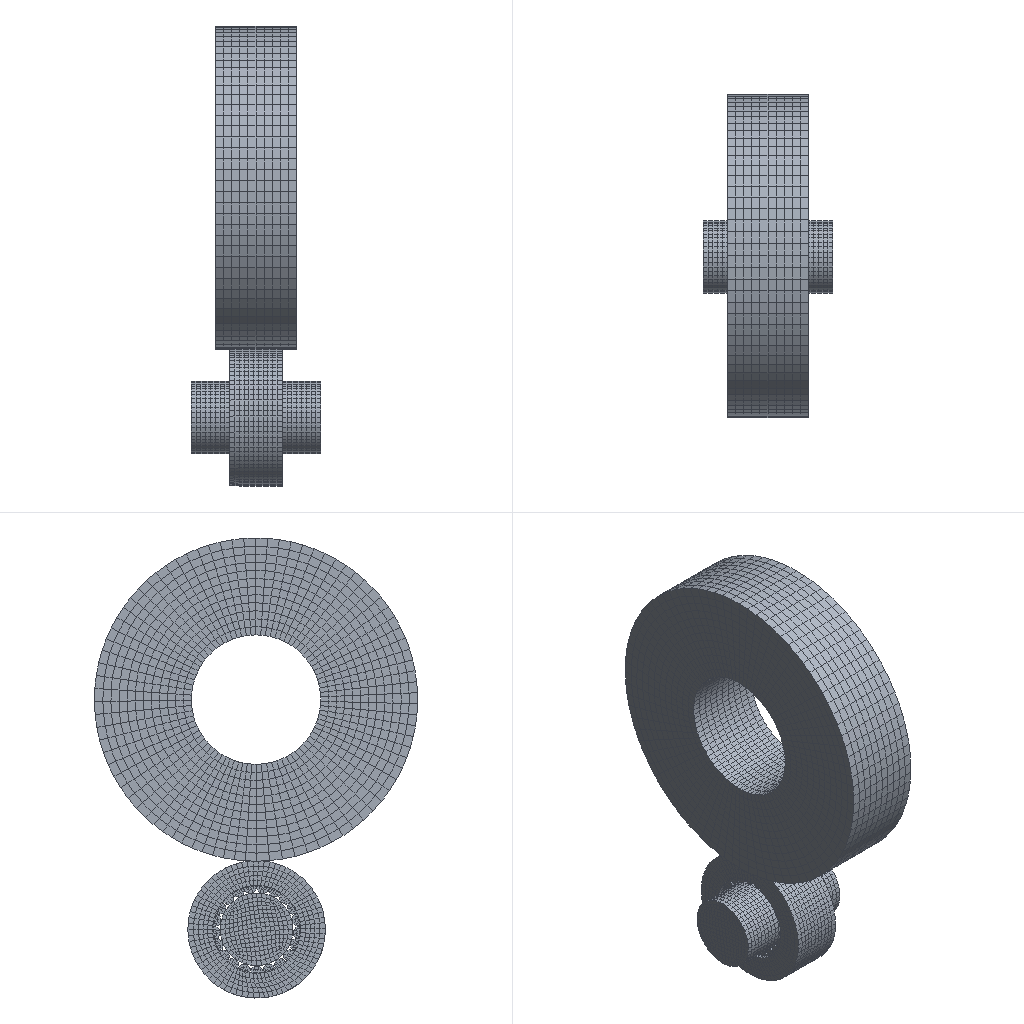Simulation study | abaqus
Set-up summary:
category,name,step,type,value,unit,region
solver,abaqus
solver,version,,,Abaqus/Explicit 2020
units,not stated in the deck,,not stated
analysis,deck,,transient,transient
load_step,Step-1,Step-1,transient
load_step,requested,,,1
mesh,nodes,,,28916
mesh,elements,,,23080
element_type,C3D8R,,solid,23080
load,load commands in deck,,count,3
bc,support commands in deck,,count,13
material,MATERIAL-1,,in results
check,setup vs results,,match,"per instance, exact: element labels, types and connectivity; labels of the nodes the elements use; coordinates of those nodes at SINGLE_PRECISION in 24 of 24 instance(s)"
Abaqus input file, long lists of numbers shortened:
*Heading
** Job name: Job-1 Model name: Model-1
** Generated by: Abaqus/CAE 2020
*Preprint, echo=NO, model=NO, history=NO, contact=NO
**
** PARTS
**
*Part, name=work-1
*Node
      1,  -7.421,    98.793,  -140.361
      2,  -7.421,   99.389,  -144.043
** (218 more lines like these left out)
*Element, type=C3D8R
  1,  17,   7,   1,   6,  39,  29,  23,  28
  2,  17,   8,   2,   7,  39,  30,  24,  29
** (142 more lines like these left out)
*Nset, nset=Set-2, generate
   1,  220,    1
*Elset, elset=Set-2, generate
   1,  144,    1
** Section: Section-1
*Solid Section, elset=Set-2, material=Material-1
,
*End Part
**
*Part, name=work-2
*Node
      1,  -7.421,   127.968,  -119.26
      2,  -7.421,   124.847,   -118.703
** (4862 more lines like these left out)
*Element, type=C3D8R
  1,   86,  140,  139,   87, 1088,  382,  383, 1089
  2,   85,  141,  140,   86, 1087,  381,  382, 1088
** (3494 more lines like these left out)
*Nset, nset=Set-2, generate
    1,  4864,     1
*Elset, elset=Set-2, generate
    1,  3496,     1
** Section: Section-1
*Solid Section, elset=Set-2, material=Material-1
,
*End Part
**
*Part, name=work-3
*Node
      1,  -7.421,   90.453,   -143.093
      2,  -7.421,    90.968,  -139.399
** (218 more lines like these left out)
*Element, type=C3D8R
  1,  17,  18,   7,   6,  39,  40,  29,  28
  2,  18,   8,   1,   7,  40,  30,  23,  29
** (142 more lines like these left out)
*Nset, nset=Set-2, generate
   1,  220,    1
*Elset, elset=Set-2, generate
   1,  144,    1
** Section: Section-1
*Solid Section, elset=Set-2, material=Material-1
,
*End Part
**
*Part, name=work-4
*Node
      1,  -7.421,   82.194,  -139.552
      2,  -7.421,   83.775,  -136.174
** (218 more lines like these left out)
*Element, type=C3D8R
  1,  17,  18,   7,   6,  39,  40,  29,  28
  2,  18,   8,   1,   7,  40,  30,  23,  29
** (142 more lines like these left out)
*Nset, nset=Set-2, generate
   1,  220,    1
*Elset, elset=Set-2, generate
   1,  144,    1
** Section: Section-1
*Solid Section, elset=Set-2, material=Material-1
,
*End Part
**
*Part, name=work-5
*Node
      1,  -7.421,   75.345,  -133.734
      2,  -7.421,   77.852,  -130.972
** (218 more lines like these left out)
*Element, type=C3D8R
  1,  17,  18,   7,   6,  39,  40,  29,  28
  2,  18,   8,   1,   7,  40,  30,  23,  29
** (142 more lines like these left out)
*Nset, nset=Set-2, generate
   1,  220,    1
*Elset, elset=Set-2, generate
   1,  144,    1
** Section: Section-1
*Solid Section, elset=Set-2, material=Material-1
,
*End Part
**
*Part, name=work-6
*Node
      1,  -7.421,   73.153,  -122.789
      2,  -7.421,   69.504,   -123.541
** (218 more lines like these left out)
*Element, type=C3D8R
  1,  17,  18,   7,   6,  39,  40,  29,  28
  2,  18,   8,   1,   7,  40,  30,  23,  29
** (142 more lines like these left out)
*Nset, nset=Set-2, generate
   1,  220,    1
*Elset, elset=Set-2, generate
   1,  144,    1
** Section: Section-1
*Solid Section, elset=Set-2, material=Material-1
,
*End Part
**
*Part, name=work-7
*Node
      1,  -7.421,   68.134,  -117.49
      2,  -7.421,   71.761,  -116.62
** (218 more lines like these left out)
*Element, type=C3D8R
  1,  17,  18,   7,   6,  39,  40,  29,  28
  2,  18,   8,   1,   7,  40,  30,  23,  29
** (142 more lines like these left out)
*Nset, nset=Set-2, generate
   1,  220,    1
*Elset, elset=Set-2, generate
   1,  144,    1
** Section: Section-1
*Solid Section, elset=Set-2, material=Material-1
,
*End Part
**
*Part, name=work-8
*Node
      1,  -7.421,   68.413,  -108.508
      2,  -7.421,   72.135,  -108.746
** (218 more lines like these left out)
*Element, type=C3D8R
  1,  17,  18,   7,   6,  39,  40,  29,  28
  2,  18,   8,   1,   7,  40,  30,  23,  29
** (142 more lines like these left out)
*Nset, nset=Set-2, generate
   1,  220,    1
*Elset, elset=Set-2, generate
   1,  144,    1
** Section: Section-1
*Solid Section, elset=Set-2, material=Material-1
,
*End Part
**
*Part, name=work-9
*Node
      1,  -7.421,   75.604,  -99.97
      2,  -7.421,   72.741,  -97.586
** (218 more lines like these left out)
*Element, type=C3D8R
  1,  17,  18,   7,   6,  39,  40,  29,  28
  2,  18,   8,   1,   7,  40,  30,  23,  29
** (142 more lines like these left out)
*Nset, nset=Set-2, generate
   1,  220,    1
*Elset, elset=Set-2, generate
   1,  144,    1
** Section: Section-1
*Solid Section, elset=Set-2, material=Material-1
,
*End Part
**
*Part, name=work-10
*Node
      1,  -7.421,   76.617,  -92.743
      2,  -7.421,   79.559,  -95.036
** (218 more lines like these left out)
*Element, type=C3D8R
  1,  17,  18,   7,   6,  39,  40,  29,  28
  2,  18,   8,   1,   7,  40,  30,  23,  29
** (142 more lines like these left out)
*Nset, nset=Set-2, generate
   1,  220,    1
*Elset, elset=Set-2, generate
   1,  144,    1
** Section: Section-1
*Solid Section, elset=Set-2, material=Material-1
,
*End Part
**
*Part, name=work-11
*Node
      1,  -7.421,   87.368,  -89.739
      2,  -7.421,   86.346,  -86.156
** (218 more lines like these left out)
*Element, type=C3D8R
  1,  17,  18,   7,   6,  39,  40,  29,  28
  2,  18,   8,   1,   7,  40,  30,  23,  29
** (142 more lines like these left out)
*Nset, nset=Set-2, generate
   1,  220,    1
*Elset, elset=Set-2, generate
   1,  144,    1
** Section: Section-1
*Solid Section, elset=Set-2, material=Material-1
,
*End Part
**
*Part, name=work-12
*Node
      1,  -7.421,   94.972,  -87.659
      2,  -7.421,   95.051,  -83.934
** (218 more lines like these left out)
*Element, type=C3D8R
  1,  17,  18,   7,   6,  39,  40,  29,  28
  2,  18,   8,   1,   7,  40,  30,  23,  29
** (142 more lines like these left out)
*Nset, nset=Set-2, generate
   1,  220,    1
*Elset, elset=Set-2, generate
   1,  144,    1
** Section: Section-1
*Solid Section, elset=Set-2, material=Material-1
,
*End Part
**
*Part, name=work-13
*Node
      1,  -7.421,   102.852,  -87.913
      2,  -7.421,   104.025,  -84.377
** (218 more lines like these left out)
*Element, type=C3D8R
  1,  17,  18,   7,   6,  39,  40,  29,  28
  2,  18,   8,   1,   7,  40,  30,  23,  29
** (142 more lines like these left out)
*Nset, nset=Set-2, generate
   1,  220,    1
*Elset, elset=Set-2, generate
   1,  144,    1
** Section: Section-1
*Solid Section, elset=Set-2, material=Material-1
,
*End Part
**
*Part, name=work-14
*Node
      1,  -7.421,   109.95,  -86.216
      2,  -7.421,   108.89,  -89.792
** (218 more lines like these left out)
*Element, type=C3D8R
  1,  17,  18,   7,   6,  39,  40,  29,  28
  2,  18,   8,   1,   7,  40,  30,  23,  29
** (142 more lines like these left out)
*Nset, nset=Set-2, generate
   1,  220,    1
*Elset, elset=Set-2, generate
   1,  144,    1
** Section: Section-1
*Solid Section, elset=Set-2, material=Material-1
,
*End Part
**
*Part, name=work-15
*Node
      1,  -7.421,   117.589,  -90.948
      2,  -7.421,   115.522,  -94.053
** (218 more lines like these left out)
*Element, type=C3D8R
  1,  17,  18,   7,   6,  39,  40,  29,  28
  2,  18,   8,   1,   7,  40,  30,  23,  29
** (142 more lines like these left out)
*Nset, nset=Set-2, generate
   1,  220,    1
*Elset, elset=Set-2, generate
   1,  144,    1
** Section: Section-1
*Solid Section, elset=Set-2, material=Material-1
,
*End Part
**
*Part, name=work-16
*Node
      1,  -7.421,   121.387,  -101.445
      2,  -7.421,   124.884,  -100.157
** (218 more lines like these left out)
*Element, type=C3D8R
  1,  17,  18,   7,   6,  39,  40,  29,  28
  2,  18,   8,   1,   7,  40,  30,  23,  29
** (142 more lines like these left out)
*Nset, nset=Set-2, generate
   1,  220,    1
*Elset, elset=Set-2, generate
   1,  144,    1
** Section: Section-1
*Solid Section, elset=Set-2, material=Material-1
,
*End Part
**
*Part, name=work-17
*Node
      1,  -7.421,   124.03,  -108.872
      2,  -7.421,    127.75,   -108.672
** (218 more lines like these left out)
*Element, type=C3D8R
  1,  17,  18,   7,   6,  39,  40,  29,  28
  2,  18,   8,   1,   7,  40,  30,  23,  29
** (142 more lines like these left out)
*Nset, nset=Set-2, generate
   1,  220,    1
*Elset, elset=Set-2, generate
   1,  144,    1
** Section: Section-1
*Solid Section, elset=Set-2, material=Material-1
,
*End Part
**
*Part, name=work-18
*Node
      1,  -7.421,   128.203,   -114.859
      2,  -7.421,   124.487,  -115.179
** (218 more lines like these left out)
*Element, type=C3D8R
  1,  17,  18,   7,   6,  39,  40,  29,  28
  2,  18,   8,   1,   7,  40,  30,  23,  29
** (142 more lines like these left out)
*Nset, nset=Set-2, generate
   1,  220,    1
*Elset, elset=Set-2, generate
   1,  144,    1
** Section: Section-1
*Solid Section, elset=Set-2, material=Material-1
,
*End Part
**
*Part, name=work-19
*Node
      1,  -7.421,   126.589,  -123.7
      2,  -7.421,    122.944,  -122.91
** (218 more lines like these left out)
*Element, type=C3D8R
  1,  17,  18,   7,   6,  39,  40,  29,  28
  2,  18,   8,   1,   7,  40,  30,  23,  29
** (142 more lines like these left out)
*Nset, nset=Set-2, generate
   1,  220,    1
*Elset, elset=Set-2, generate
   1,  144,    1
** Section: Section-1
*Solid Section, elset=Set-2, material=Material-1
,
*End Part
**
*Part, name=work-20
*Node
      1,  -7.421,   122.44,  -131.671
      2,  -7.421,   119.19,  -129.842
** (218 more lines like these left out)
*Element, type=C3D8R
  1,  17,  18,   7,   6,  39,  40,  29,  28
  2,  18,   8,   1,   7,  40,  30,  23,  29
** (142 more lines like these left out)
*Nset, nset=Set-2, generate
   1,  220,    1
*Elset, elset=Set-2, generate
   1,  144,    1
** Section: Section-1
*Solid Section, elset=Set-2, material=Material-1
,
*End Part
**
*Part, name=work-21
*Node
      1,  -7.421,   116.127,  -138.066
      2,  -7.421,   113.56,  -135.36
** (218 more lines like these left out)
*Element, type=C3D8R
  1,  17,  18,   7,   6,  39,  40,  29,  28
  2,  18,   8,   1,   7,  40,  30,  23,  29
** (142 more lines like these left out)
*Nset, nset=Set-2, generate
   1,  220,    1
*Elset, elset=Set-2, generate
   1,  144,    1
** Section: Section-1
*Solid Section, elset=Set-2, material=Material-1
,
*End Part
**
*Part, name=work-22
*Node
      1,  -7.421,    106.553,  -138.973
      2,  -7.421,   108.208,  -142.316
** (218 more lines like these left out)
*Element, type=C3D8R
  1,  17,   7,   1,   6,  39,  29,  23,  28
  2,  17,   8,   2,   7,  39,  30,  24,  29
** (142 more lines like these left out)
*Nset, nset=Set-2, generate
   1,  220,    1
*Elset, elset=Set-2, generate
   1,  144,    1
** Section: Section-1
*Solid Section, elset=Set-2, material=Material-1
,
*End Part
**
*Part, name=work-23
*Node
      1,   19.579,   98.623,  -109.942
      2,   19.579,   76.403,  -107.859
** (7418 more lines like these left out)
*Element, type=C3D8R
   1,   89,   91,    8,    7,  354,  356,  273,  272
   2,   91,   92,    9,    8,  356,  357,  274,  273
** (6478 more lines like these left out)
*Nset, nset=Set-2, generate
    1,  7420,     1
*Elset, elset=Set-2, generate
    1,  6480,     1
** Section: Section-1
*Solid Section, elset=Set-2, material=Material-1
,
*End Part
**
*Part, name=work-24
*Node
      1,  -45.421,   60.427,   41.094
      2,  -45.421,   3.444,   59.882
** (12010 more lines like these left out)
*Element, type=C3D8R
    1,    66,   235,    13,     1,  1158,  1327,  1105,  1093
    2,   235,   236,    14,    13,  1327,  1328,  1106,  1105
** (10078 more lines like these left out)
*Nset, nset=Set-2, generate
     1,  12012,      1
*Elset, elset=Set-2, generate
     1,  10080,      1
** Section: Section-1
*Solid Section, elset=Set-2, material=Material-1
,
*End Part
**
**
** ASSEMBLY
**
*Assembly, name=Assembly
**
*Instance, name=work-1-1, part=work-1
*End Instance
**
*Instance, name=work-2-1, part=work-2
*End Instance
**
*Instance, name=work-3-1, part=work-3
*End Instance
**
*Instance, name=work-4-1, part=work-4
*End Instance
**
*Instance, name=work-5-1, part=work-5
*End Instance
**
*Instance, name=work-6-1, part=work-6
*End Instance
**
*Instance, name=work-7-1, part=work-7
*End Instance
**
*Instance, name=work-8-1, part=work-8
*End Instance
**
*Instance, name=work-9-1, part=work-9
*End Instance
**
*Instance, name=work-10-1, part=work-10
*End Instance
**
*Instance, name=work-11-1, part=work-11
*End Instance
**
*Instance, name=work-12-1, part=work-12
*End Instance
**
*Instance, name=work-13-1, part=work-13
*End Instance
**
*Instance, name=work-14-1, part=work-14
*End Instance
**
*Instance, name=work-15-1, part=work-15
*End Instance
**
*Instance, name=work-16-1, part=work-16
*End Instance
**
*Instance, name=work-17-1, part=work-17
*End Instance
**
*Instance, name=work-18-1, part=work-18
*End Instance
**
*Instance, name=work-19-1, part=work-19
*End Instance
**
*Instance, name=work-20-1, part=work-20
*End Instance
**
*Instance, name=work-21-1, part=work-21
*End Instance
**
*Instance, name=work-22-1, part=work-22
*End Instance
**
*Instance, name=work-23-1, part=work-23
*End Instance
**
*Instance, name=work-24-1, part=work-24
          0.,           0.,         -0.3
*End Instance
**
*Node
      1,  -20.421,   98.417,   28.276
*Node
      2,  -20.421,   98.07,  -113.924
*Node
      3,  -4.171,   98.07,  -113.924
*Nset, nset=Set-3
 1,
*Nset, nset=Set-4
 2,
*Nset, nset=Set-5
 2,
*Nset, nset=Set-6
 2,
*Nset, nset=Set-8
 3,
*Nset, nset=m_Set-1
 1,
*Nset, nset=m_Set-2
 2,
*Nset, nset=m_Set-7
 3,
*Elset, elset=_m_Surf-1_S6, internal, instance=work-24-1
  337,  349,  361,  373,  385,  397,  409,  421,  433,  445,  457,  469,  481,  493,  505,  517
  529,  541,  553,  565,  577,  589,  601,  613,  625,  637,  649,  661,  673,  685,  697,  709
** (27 more lines like these left out)
*Elset, elset=_m_Surf-1_S4, internal, instance=work-24-1
    12,    24,    36,    48,    60,    72,    84,    96,   108,   120,   132,   144,   156,   168,   180,   192
   204,   216,   228,   240,   252,   264,   276,   288,   300,   312,   324,   336,   888,   900,   912,   924
** (23 more lines like these left out)
*Surface, type=ELEMENT, name=m_Surf-1
_m_Surf-1_S6, S6
_m_Surf-1_S4, S4
*Elset, elset=_s_Surf-1_S3, internal, instance=work-2-1
  489,  493,  497,  501,  505,  509,  513,  517,  521,  525,  529,  533,  537,  541,  545,  549
  553,  557,  561,  565,  569,  573,  577,  581,  585,  589,  593,  597,  601,  793,  797,  801
** (17 more lines like these left out)
*Elset, elset=_s_Surf-1_S5, internal, instance=work-2-1
  384,  388,  392,  396,  400,  404,  408,  412,  416,  420,  424,  428,  432,  436,  440,  444
  448,  452,  456,  460,  464,  468,  472,  476,  480,  484,  488,  608,  612,  616,  620,  624
** (28 more lines like these left out)
*Elset, elset=_s_Surf-1_S6, internal, instance=work-2-1, generate
 185,  297,    4
*Elset, elset=_s_Surf-1_S4, internal, instance=work-2-1
  80,  84,  88,  92,  96, 100, 104, 108, 112, 116, 120, 124, 128, 132, 136, 140
 144, 148, 152, 156, 160, 164, 168, 172, 176, 180, 184, 304, 308, 312, 316, 320
** (1 more lines like these left out)
*Surface, type=ELEMENT, name=s_Surf-1
_s_Surf-1_S3, S3
_s_Surf-1_S5, S5
_s_Surf-1_S6, S6
_s_Surf-1_S4, S4
*Elset, elset=_s_Surf-3_S6, internal, instance=work-24-1
     1,    13,    25,    37,    49,    61,    73,    85,    97,   109,   121,   133,   145,   157,   169,   181
   193,   205,   217,   229,   241,   253,   265,   277,   289,   301,   313,   325,   877,   889,   901,   913
** (23 more lines like these left out)
*Elset, elset=_s_Surf-3_S4, internal, instance=work-24-1
  348,  360,  372,  384,  396,  408,  420,  432,  444,  456,  468,  480,  492,  504,  516,  528
  540,  552,  564,  576,  588,  600,  612,  624,  636,  648,  660,  672,  684,  696,  708,  720
** (27 more lines like these left out)
*Elset, elset=_s_Surf-3_S2, internal, instance=work-24-1, generate
  9073,  10080,      1
*Elset, elset=_s_Surf-3_S1, internal, instance=work-24-1, generate
    1,  1008,     1
*Surface, type=ELEMENT, name=s_Surf-3
_s_Surf-3_S6, S6
_s_Surf-3_S4, S4
_s_Surf-3_S2, S2
_s_Surf-3_S1, S1
*Elset, elset=_s_Surf-4_S2, internal, instance=work-23-1, generate
 6241,  6480,     1
*Elset, elset=_s_Surf-4_S1, internal, instance=work-23-1, generate
   1,  240,    1
*Surface, type=ELEMENT, name=s_Surf-4
_s_Surf-4_S2, S2
_s_Surf-4_S1, S1
*Elset, elset=_s_Surf-5_S6, internal, instance=work-24-1
     1,    13,    25,    37,    49,    61,    73,    85,    97,   109,   121,   133,   145,   157,   169,   181
   193,   205,   217,   229,   241,   253,   265,   277,   289,   301,   313,   325,   877,   889,   901,   913
** (23 more lines like these left out)
*Elset, elset=_s_Surf-5_S4, internal, instance=work-24-1
  348,  360,  372,  384,  396,  408,  420,  432,  444,  456,  468,  480,  492,  504,  516,  528
  540,  552,  564,  576,  588,  600,  612,  624,  636,  648,  660,  672,  684,  696,  708,  720
** (27 more lines like these left out)
*Surface, type=ELEMENT, name=s_Surf-5
_s_Surf-5_S6, S6
_s_Surf-5_S4, S4
*Elset, elset=_s_Surf-6_S2, internal, instance=work-2-1
    1,    2,    3,    4,    5,    6,    7,    8,    9,   10,   11,   12,   13,   14,   15,   16
   17,   18,   19,   20,   21,   22,   23,   24,   25,   26,   27,   28,   29,   30,   31,   32
** (46 more lines like these left out)
*Surface, type=ELEMENT, name=s_Surf-6
_s_Surf-6_S2, S2
** Constraint: Constraint-1
*Coupling, constraint name=Constraint-1, ref node=m_Set-1, surface=s_Surf-5
*Kinematic
** Constraint: Constraint-2
*Coupling, constraint name=Constraint-2, ref node=m_Set-2, surface=s_Surf-4
*Kinematic
** Constraint: Constraint-3
*Coupling, constraint name=Constraint-3, ref node=m_Set-7, surface=s_Surf-6
*Kinematic
*End Assembly
**
** MATERIALS
**
*Material, name=Material-1
*Density
 7.8e-09,
*Elastic
210000., 0.3
**
** INTERACTION PROPERTIES
**
*Surface Interaction, name=IntProp-1
*Friction
 0.3,
*Surface Behavior, pressure-overclosure=HARD
** ----------------------------------------------------------------
**
** STEP: Step-1
**
*Step, name=Step-1, nlgeom=YES
*Dynamic, Explicit
, 0.1
*Bulk Viscosity
0.06, 1.2
**
** BOUNDARY CONDITIONS
**
** Name: BC-1 Type: 位移/转角
*Boundary
Set-3, 1, 1
Set-3, 2, 2
Set-3, 3, 3
Set-3, 5, 5
Set-3, 6, 6
** Name: BC-2 Type: 位移/转角
*Boundary
Set-6, 1, 1
Set-6, 5, 5
Set-6, 6, 6
** Name: BC-3 Type: 位移/转角
*Boundary
Set-8, 1, 1
Set-8, 2, 2
Set-8, 3, 3
Set-8, 5, 5
Set-8, 6, 6
**
** LOADS
**
** Name: Load-1   Type: Concentrated force
*Cload
Set-4, 2, 0.
Set-4, 3, 100000.
** Name: Load-2   Type: Moment
*Cload
Set-5, 4, 500000.
**
** INTERACTIONS
**
** Interaction: Int-1
*Contact Pair, interaction=IntProp-1, mechanical constraint=KINEMATIC, cpset=Int-1
m_Surf-1, s_Surf-1
** Interaction: Int-2
*Contact, op=NEW
*Contact Inclusions, ALL EXTERIOR
*Contact Property Assignment
 ,  , IntProp-1
**
** OUTPUT REQUESTS
**
*Restart, write, number interval=1, time marks=NO
**
** FIELD OUTPUT: F-Output-1
**
*Output, field, number interval=50
*Node Output
A, CF, RF, RM, RT, U, UR, UT
V, VR, VT
*Element Output, directions=YES
E, EVF, LE, MISES, MISESMAX, PE, PEEQ, PEEQVAVG, PEVAVG, S, SF, SVAVG, VE
*Contact Output
CDISP, CSTRESS
**
** HISTORY OUTPUT: H-Output-1
**
*Output, history, variable=PRESELECT
*End Step
Results summary:
result,step,Step-1,partial,increments=78409 time=0.01682/0.1
result,analysis,,,transient
result,last_loadstep,,,1
result,primary field,,,U
result,reaction total,,FX,-34429.026,model units
result,reaction total,,FY,-60299.57,model units
result,reaction total,,FZ,74531.219,model units